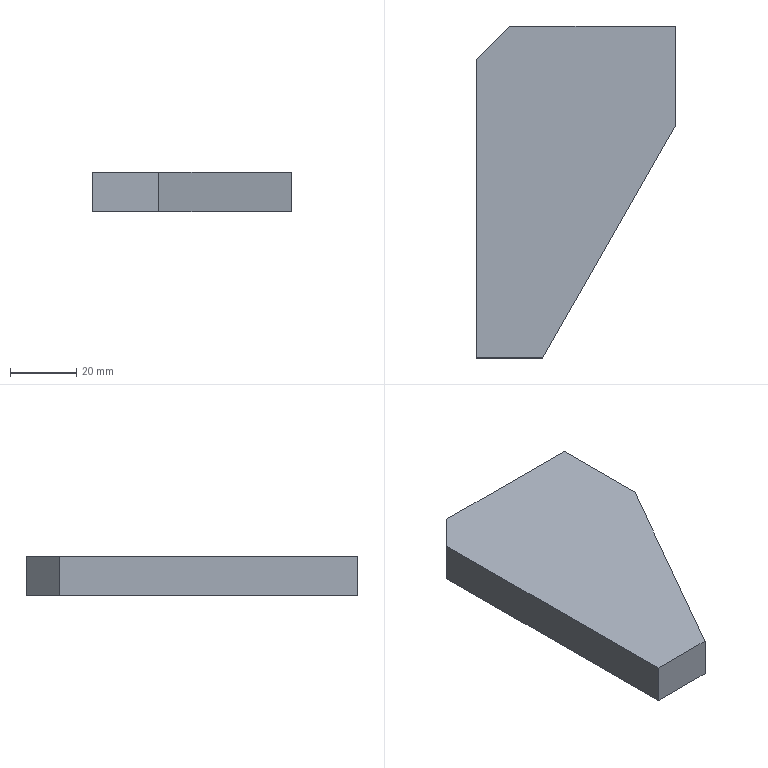Part | STEP file | Gusset plate 1_Default<As machined> | 1 solid | 8 faces | box 60 x 100 x 12 mm | volume 54600 mm3 | plane 8
STEP:
#1=CARTESIAN_POINT('',(0.,0.,0.));
#2=DIRECTION('',(0.,0.,1.));
#3=DIRECTION('',(1.,0.,0.));
#4=AXIS2_PLACEMENT_3D('',#1,#2,#3);
#5=CARTESIAN_POINT('',(0.,-100.,-6.));
#6=VERTEX_POINT('',#5);
#7=CARTESIAN_POINT('',(20.,-100.,-6.));
#8=VERTEX_POINT('',#7);
#9=CARTESIAN_POINT('',(0.,-100.,-6.));
#10=DIRECTION('',(1.,0.,0.));
#11=VECTOR('',#10,1.);
#12=LINE('',#9,#11);
#13=CARTESIAN_POINT('',(0.,-100.,6.));
#14=DIRECTION('',(0.,1.,0.));
#15=DIRECTION('',(0.,0.,1.));
#16=AXIS2_PLACEMENT_3D('',#13,#14,#15);
#17=PLANE('',#16);
#18=CARTESIAN_POINT('',(-12.,0.));
#19=DIRECTION('',(0.,1.));
#20=VECTOR('',#19,1.);
#21=LINE('',#18,#20);
#22=(GEOMETRIC_REPRESENTATION_CONTEXT(2)PARAMETRIC_REPRESENTATION_CONTEXT()REPRESENTATION_CONTEXT('',''));
#23=DEFINITIONAL_REPRESENTATION('',(#21),#22);
#24=PCURVE('',#17,#23);
#25=CARTESIAN_POINT('',(0.,0.,-6.));
#26=DIRECTION('',(0.,0.,1.));
#27=DIRECTION('',(1.,0.,0.));
#28=AXIS2_PLACEMENT_3D('',#25,#26,#27);
#29=PLANE('',#28);
#30=CARTESIAN_POINT('',(0.,-100.));
#31=DIRECTION('',(1.,0.));
#32=VECTOR('',#31,1.);
#33=LINE('',#30,#32);
#34=(GEOMETRIC_REPRESENTATION_CONTEXT(2)PARAMETRIC_REPRESENTATION_CONTEXT()REPRESENTATION_CONTEXT('',''));
#35=DEFINITIONAL_REPRESENTATION('',(#33),#34);
#36=PCURVE('',#29,#35);
#37=SURFACE_CURVE('',#12,(#24,#36),.PCURVE_S1.);
#38=EDGE_CURVE('',#6,#8,#37,.T.);
#39=ORIENTED_EDGE('',*,*,#38,.T.);
#40=CARTESIAN_POINT('',(20.,-100.,6.));
#41=VERTEX_POINT('',#40);
#42=CARTESIAN_POINT('',(20.,-100.,6.));
#43=DIRECTION('',(0.,0.,-1.));
#44=VECTOR('',#43,1.);
#45=LINE('',#42,#44);
#46=CARTESIAN_POINT('',(0.,20.));
#47=DIRECTION('',(-1.,0.));
#48=VECTOR('',#47,1.);
#49=LINE('',#46,#48);
#50=(GEOMETRIC_REPRESENTATION_CONTEXT(2)PARAMETRIC_REPRESENTATION_CONTEXT()REPRESENTATION_CONTEXT('',''));
#51=DEFINITIONAL_REPRESENTATION('',(#49),#50);
#52=PCURVE('',#17,#51);
#53=CARTESIAN_POINT('',(20.,-100.,6.));
#54=DIRECTION('',(-0.8682,0.4961,0.));
#55=DIRECTION('',(-0.4961,-0.8682,0.));
#56=AXIS2_PLACEMENT_3D('',#53,#54,#55);
#57=PLANE('',#56);
#58=CARTESIAN_POINT('',(0.,0.));
#59=DIRECTION('',(0.,-1.));
#60=VECTOR('',#59,1.);
#61=LINE('',#58,#60);
#62=(GEOMETRIC_REPRESENTATION_CONTEXT(2)PARAMETRIC_REPRESENTATION_CONTEXT()REPRESENTATION_CONTEXT('',''));
#63=DEFINITIONAL_REPRESENTATION('',(#61),#62);
#64=PCURVE('',#57,#63);
#65=SURFACE_CURVE('',#45,(#52,#64),.PCURVE_S1.);
#66=EDGE_CURVE('',#41,#8,#65,.T.);
#67=ORIENTED_EDGE('',*,*,#66,.F.);
#68=CARTESIAN_POINT('',(0.,-100.,6.));
#69=VERTEX_POINT('',#68);
#70=CARTESIAN_POINT('',(0.,-100.,6.));
#71=DIRECTION('',(1.,0.,0.));
#72=VECTOR('',#71,1.);
#73=LINE('',#70,#72);
#74=CARTESIAN_POINT('',(0.,0.));
#75=DIRECTION('',(0.,1.));
#76=VECTOR('',#75,1.);
#77=LINE('',#74,#76);
#78=(GEOMETRIC_REPRESENTATION_CONTEXT(2)PARAMETRIC_REPRESENTATION_CONTEXT()REPRESENTATION_CONTEXT('',''));
#79=DEFINITIONAL_REPRESENTATION('',(#77),#78);
#80=PCURVE('',#17,#79);
#81=CARTESIAN_POINT('',(0.,0.,6.));
#82=DIRECTION('',(0.,0.,1.));
#83=DIRECTION('',(1.,0.,0.));
#84=AXIS2_PLACEMENT_3D('',#81,#82,#83);
#85=PLANE('',#84);
#86=CARTESIAN_POINT('',(0.,-100.));
#87=DIRECTION('',(1.,0.));
#88=VECTOR('',#87,1.);
#89=LINE('',#86,#88);
#90=(GEOMETRIC_REPRESENTATION_CONTEXT(2)PARAMETRIC_REPRESENTATION_CONTEXT()REPRESENTATION_CONTEXT('',''));
#91=DEFINITIONAL_REPRESENTATION('',(#89),#90);
#92=PCURVE('',#85,#91);
#93=SURFACE_CURVE('',#73,(#80,#92),.PCURVE_S1.);
#94=EDGE_CURVE('',#69,#41,#93,.T.);
#95=ORIENTED_EDGE('',*,*,#94,.F.);
#96=CARTESIAN_POINT('',(0.,-100.,6.));
#97=DIRECTION('',(0.,0.,-1.));
#98=VECTOR('',#97,1.);
#99=LINE('',#96,#98);
#100=CARTESIAN_POINT('',(0.,0.));
#101=DIRECTION('',(-1.,0.));
#102=VECTOR('',#101,1.);
#103=LINE('',#100,#102);
#104=(GEOMETRIC_REPRESENTATION_CONTEXT(2)PARAMETRIC_REPRESENTATION_CONTEXT()REPRESENTATION_CONTEXT('',''));
#105=DEFINITIONAL_REPRESENTATION('',(#103),#104);
#106=PCURVE('',#17,#105);
#107=CARTESIAN_POINT('',(0.,-10.,6.));
#108=DIRECTION('',(1.,0.,0.));
#109=DIRECTION('',(0.,1.,0.));
#110=AXIS2_PLACEMENT_3D('',#107,#108,#109);
#111=PLANE('',#110);
#112=CARTESIAN_POINT('',(-90.,0.));
#113=DIRECTION('',(0.,-1.));
#114=VECTOR('',#113,1.);
#115=LINE('',#112,#114);
#116=(GEOMETRIC_REPRESENTATION_CONTEXT(2)PARAMETRIC_REPRESENTATION_CONTEXT()REPRESENTATION_CONTEXT('',''));
#117=DEFINITIONAL_REPRESENTATION('',(#115),#116);
#118=PCURVE('',#111,#117);
#119=SURFACE_CURVE('',#99,(#106,#118),.PCURVE_S1.);
#120=EDGE_CURVE('',#69,#6,#119,.T.);
#121=ORIENTED_EDGE('',*,*,#120,.T.);
#122=EDGE_LOOP('',(#39,#67,#95,#121));
#123=FACE_BOUND('',#122,.T.);
#124=ADVANCED_FACE('',(#123),#17,.F.);
#125=CARTESIAN_POINT('',(60.,-30.,-6.));
#126=VERTEX_POINT('',#125);
#127=CARTESIAN_POINT('',(20.,-100.,-6.));
#128=DIRECTION('',(0.4961,0.8682,0.));
#129=VECTOR('',#128,1.);
#130=LINE('',#127,#129);
#131=CARTESIAN_POINT('',(0.,-12.));
#132=DIRECTION('',(-1.,0.));
#133=VECTOR('',#132,1.);
#134=LINE('',#131,#133);
#135=(GEOMETRIC_REPRESENTATION_CONTEXT(2)PARAMETRIC_REPRESENTATION_CONTEXT()REPRESENTATION_CONTEXT('',''));
#136=DEFINITIONAL_REPRESENTATION('',(#134),#135);
#137=PCURVE('',#57,#136);
#138=CARTESIAN_POINT('',(20.,-100.));
#139=DIRECTION('',(0.4961,0.8682));
#140=VECTOR('',#139,1.);
#141=LINE('',#138,#140);
#142=(GEOMETRIC_REPRESENTATION_CONTEXT(2)PARAMETRIC_REPRESENTATION_CONTEXT()REPRESENTATION_CONTEXT('',''));
#143=DEFINITIONAL_REPRESENTATION('',(#141),#142);
#144=PCURVE('',#29,#143);
#145=SURFACE_CURVE('',#130,(#137,#144),.PCURVE_S1.);
#146=EDGE_CURVE('',#8,#126,#145,.T.);
#147=ORIENTED_EDGE('',*,*,#146,.T.);
#148=CARTESIAN_POINT('',(60.,-30.,6.));
#149=VERTEX_POINT('',#148);
#150=CARTESIAN_POINT('',(60.,-30.,6.));
#151=DIRECTION('',(0.,0.,-1.));
#152=VECTOR('',#151,1.);
#153=LINE('',#150,#152);
#154=CARTESIAN_POINT('',(-80.623,0.));
#155=DIRECTION('',(0.,-1.));
#156=VECTOR('',#155,1.);
#157=LINE('',#154,#156);
#158=(GEOMETRIC_REPRESENTATION_CONTEXT(2)PARAMETRIC_REPRESENTATION_CONTEXT()REPRESENTATION_CONTEXT('',''));
#159=DEFINITIONAL_REPRESENTATION('',(#157),#158);
#160=PCURVE('',#57,#159);
#161=CARTESIAN_POINT('',(60.,-30.,6.));
#162=DIRECTION('',(-1.,0.,0.));
#163=DIRECTION('',(0.,0.,1.));
#164=AXIS2_PLACEMENT_3D('',#161,#162,#163);
#165=PLANE('',#164);
#166=CARTESIAN_POINT('',(0.,0.));
#167=DIRECTION('',(-1.,0.));
#168=VECTOR('',#167,1.);
#169=LINE('',#166,#168);
#170=(GEOMETRIC_REPRESENTATION_CONTEXT(2)PARAMETRIC_REPRESENTATION_CONTEXT()REPRESENTATION_CONTEXT('',''));
#171=DEFINITIONAL_REPRESENTATION('',(#169),#170);
#172=PCURVE('',#165,#171);
#173=SURFACE_CURVE('',#153,(#160,#172),.PCURVE_S1.);
#174=EDGE_CURVE('',#149,#126,#173,.T.);
#175=ORIENTED_EDGE('',*,*,#174,.F.);
#176=CARTESIAN_POINT('',(20.,-100.,6.));
#177=DIRECTION('',(0.4961,0.8682,0.));
#178=VECTOR('',#177,1.);
#179=LINE('',#176,#178);
#180=CARTESIAN_POINT('',(0.,0.));
#181=DIRECTION('',(-1.,0.));
#182=VECTOR('',#181,1.);
#183=LINE('',#180,#182);
#184=(GEOMETRIC_REPRESENTATION_CONTEXT(2)PARAMETRIC_REPRESENTATION_CONTEXT()REPRESENTATION_CONTEXT('',''));
#185=DEFINITIONAL_REPRESENTATION('',(#183),#184);
#186=PCURVE('',#57,#185);
#187=CARTESIAN_POINT('',(20.,-100.));
#188=DIRECTION('',(0.4961,0.8682));
#189=VECTOR('',#188,1.);
#190=LINE('',#187,#189);
#191=(GEOMETRIC_REPRESENTATION_CONTEXT(2)PARAMETRIC_REPRESENTATION_CONTEXT()REPRESENTATION_CONTEXT('',''));
#192=DEFINITIONAL_REPRESENTATION('',(#190),#191);
#193=PCURVE('',#85,#192);
#194=SURFACE_CURVE('',#179,(#186,#193),.PCURVE_S1.);
#195=EDGE_CURVE('',#41,#149,#194,.T.);
#196=ORIENTED_EDGE('',*,*,#195,.F.);
#197=ORIENTED_EDGE('',*,*,#66,.T.);
#198=EDGE_LOOP('',(#147,#175,#196,#197));
#199=FACE_BOUND('',#198,.T.);
#200=ADVANCED_FACE('',(#199),#57,.F.);
#201=CARTESIAN_POINT('',(60.,0.,-6.));
#202=VERTEX_POINT('',#201);
#203=CARTESIAN_POINT('',(60.,-30.,-6.));
#204=DIRECTION('',(0.,1.,0.));
#205=VECTOR('',#204,1.);
#206=LINE('',#203,#205);
#207=CARTESIAN_POINT('',(-12.,0.));
#208=DIRECTION('',(0.,1.));
#209=VECTOR('',#208,1.);
#210=LINE('',#207,#209);
#211=(GEOMETRIC_REPRESENTATION_CONTEXT(2)PARAMETRIC_REPRESENTATION_CONTEXT()REPRESENTATION_CONTEXT('',''));
#212=DEFINITIONAL_REPRESENTATION('',(#210),#211);
#213=PCURVE('',#165,#212);
#214=CARTESIAN_POINT('',(60.,-30.));
#215=DIRECTION('',(0.,1.));
#216=VECTOR('',#215,1.);
#217=LINE('',#214,#216);
#218=(GEOMETRIC_REPRESENTATION_CONTEXT(2)PARAMETRIC_REPRESENTATION_CONTEXT()REPRESENTATION_CONTEXT('',''));
#219=DEFINITIONAL_REPRESENTATION('',(#217),#218);
#220=PCURVE('',#29,#219);
#221=SURFACE_CURVE('',#206,(#213,#220),.PCURVE_S1.);
#222=EDGE_CURVE('',#126,#202,#221,.T.);
#223=ORIENTED_EDGE('',*,*,#222,.T.);
#224=CARTESIAN_POINT('',(60.,0.,6.));
#225=VERTEX_POINT('',#224);
#226=CARTESIAN_POINT('',(60.,0.,6.));
#227=DIRECTION('',(0.,0.,-1.));
#228=VECTOR('',#227,1.);
#229=LINE('',#226,#228);
#230=CARTESIAN_POINT('',(0.,30.));
#231=DIRECTION('',(-1.,0.));
#232=VECTOR('',#231,1.);
#233=LINE('',#230,#232);
#234=(GEOMETRIC_REPRESENTATION_CONTEXT(2)PARAMETRIC_REPRESENTATION_CONTEXT()REPRESENTATION_CONTEXT('',''));
#235=DEFINITIONAL_REPRESENTATION('',(#233),#234);
#236=PCURVE('',#165,#235);
#237=CARTESIAN_POINT('',(60.,0.,6.));
#238=DIRECTION('',(0.,-1.,0.));
#239=DIRECTION('',(1.,0.,0.));
#240=AXIS2_PLACEMENT_3D('',#237,#238,#239);
#241=PLANE('',#240);
#242=CARTESIAN_POINT('',(0.,0.));
#243=DIRECTION('',(0.,-1.));
#244=VECTOR('',#243,1.);
#245=LINE('',#242,#244);
#246=(GEOMETRIC_REPRESENTATION_CONTEXT(2)PARAMETRIC_REPRESENTATION_CONTEXT()REPRESENTATION_CONTEXT('',''));
#247=DEFINITIONAL_REPRESENTATION('',(#245),#246);
#248=PCURVE('',#241,#247);
#249=SURFACE_CURVE('',#229,(#236,#248),.PCURVE_S1.);
#250=EDGE_CURVE('',#225,#202,#249,.T.);
#251=ORIENTED_EDGE('',*,*,#250,.F.);
#252=CARTESIAN_POINT('',(60.,-30.,6.));
#253=DIRECTION('',(0.,1.,0.));
#254=VECTOR('',#253,1.);
#255=LINE('',#252,#254);
#256=CARTESIAN_POINT('',(0.,0.));
#257=DIRECTION('',(0.,1.));
#258=VECTOR('',#257,1.);
#259=LINE('',#256,#258);
#260=(GEOMETRIC_REPRESENTATION_CONTEXT(2)PARAMETRIC_REPRESENTATION_CONTEXT()REPRESENTATION_CONTEXT('',''));
#261=DEFINITIONAL_REPRESENTATION('',(#259),#260);
#262=PCURVE('',#165,#261);
#263=CARTESIAN_POINT('',(60.,-30.));
#264=DIRECTION('',(0.,1.));
#265=VECTOR('',#264,1.);
#266=LINE('',#263,#265);
#267=(GEOMETRIC_REPRESENTATION_CONTEXT(2)PARAMETRIC_REPRESENTATION_CONTEXT()REPRESENTATION_CONTEXT('',''));
#268=DEFINITIONAL_REPRESENTATION('',(#266),#267);
#269=PCURVE('',#85,#268);
#270=SURFACE_CURVE('',#255,(#262,#269),.PCURVE_S1.);
#271=EDGE_CURVE('',#149,#225,#270,.T.);
#272=ORIENTED_EDGE('',*,*,#271,.F.);
#273=ORIENTED_EDGE('',*,*,#174,.T.);
#274=EDGE_LOOP('',(#223,#251,#272,#273));
#275=FACE_BOUND('',#274,.T.);
#276=ADVANCED_FACE('',(#275),#165,.F.);
#277=CARTESIAN_POINT('',(10.,0.,-6.));
#278=VERTEX_POINT('',#277);
#279=CARTESIAN_POINT('',(60.,0.,-6.));
#280=DIRECTION('',(-1.,0.,0.));
#281=VECTOR('',#280,1.);
#282=LINE('',#279,#281);
#283=CARTESIAN_POINT('',(0.,-12.));
#284=DIRECTION('',(-1.,0.));
#285=VECTOR('',#284,1.);
#286=LINE('',#283,#285);
#287=(GEOMETRIC_REPRESENTATION_CONTEXT(2)PARAMETRIC_REPRESENTATION_CONTEXT()REPRESENTATION_CONTEXT('',''));
#288=DEFINITIONAL_REPRESENTATION('',(#286),#287);
#289=PCURVE('',#241,#288);
#290=CARTESIAN_POINT('',(60.,0.));
#291=DIRECTION('',(-1.,0.));
#292=VECTOR('',#291,1.);
#293=LINE('',#290,#292);
#294=(GEOMETRIC_REPRESENTATION_CONTEXT(2)PARAMETRIC_REPRESENTATION_CONTEXT()REPRESENTATION_CONTEXT('',''));
#295=DEFINITIONAL_REPRESENTATION('',(#293),#294);
#296=PCURVE('',#29,#295);
#297=SURFACE_CURVE('',#282,(#289,#296),.PCURVE_S1.);
#298=EDGE_CURVE('',#202,#278,#297,.T.);
#299=ORIENTED_EDGE('',*,*,#298,.T.);
#300=CARTESIAN_POINT('',(10.,0.,6.));
#301=VERTEX_POINT('',#300);
#302=CARTESIAN_POINT('',(10.,0.,6.));
#303=DIRECTION('',(0.,0.,-1.));
#304=VECTOR('',#303,1.);
#305=LINE('',#302,#304);
#306=CARTESIAN_POINT('',(-50.,0.));
#307=DIRECTION('',(0.,-1.));
#308=VECTOR('',#307,1.);
#309=LINE('',#306,#308);
#310=(GEOMETRIC_REPRESENTATION_CONTEXT(2)PARAMETRIC_REPRESENTATION_CONTEXT()REPRESENTATION_CONTEXT('',''));
#311=DEFINITIONAL_REPRESENTATION('',(#309),#310);
#312=PCURVE('',#241,#311);
#313=CARTESIAN_POINT('',(10.,0.,6.));
#314=DIRECTION('',(0.7071,-0.7071,0.));
#315=DIRECTION('',(0.7071,0.7071,0.));
#316=AXIS2_PLACEMENT_3D('',#313,#314,#315);
#317=PLANE('',#316);
#318=CARTESIAN_POINT('',(0.,0.));
#319=DIRECTION('',(0.,-1.));
#320=VECTOR('',#319,1.);
#321=LINE('',#318,#320);
#322=(GEOMETRIC_REPRESENTATION_CONTEXT(2)PARAMETRIC_REPRESENTATION_CONTEXT()REPRESENTATION_CONTEXT('',''));
#323=DEFINITIONAL_REPRESENTATION('',(#321),#322);
#324=PCURVE('',#317,#323);
#325=SURFACE_CURVE('',#305,(#312,#324),.PCURVE_S1.);
#326=EDGE_CURVE('',#301,#278,#325,.T.);
#327=ORIENTED_EDGE('',*,*,#326,.F.);
#328=CARTESIAN_POINT('',(60.,0.,6.));
#329=DIRECTION('',(-1.,0.,0.));
#330=VECTOR('',#329,1.);
#331=LINE('',#328,#330);
#332=CARTESIAN_POINT('',(0.,0.));
#333=DIRECTION('',(-1.,0.));
#334=VECTOR('',#333,1.);
#335=LINE('',#332,#334);
#336=(GEOMETRIC_REPRESENTATION_CONTEXT(2)PARAMETRIC_REPRESENTATION_CONTEXT()REPRESENTATION_CONTEXT('',''));
#337=DEFINITIONAL_REPRESENTATION('',(#335),#336);
#338=PCURVE('',#241,#337);
#339=CARTESIAN_POINT('',(60.,0.));
#340=DIRECTION('',(-1.,0.));
#341=VECTOR('',#340,1.);
#342=LINE('',#339,#341);
#343=(GEOMETRIC_REPRESENTATION_CONTEXT(2)PARAMETRIC_REPRESENTATION_CONTEXT()REPRESENTATION_CONTEXT('',''));
#344=DEFINITIONAL_REPRESENTATION('',(#342),#343);
#345=PCURVE('',#85,#344);
#346=SURFACE_CURVE('',#331,(#338,#345),.PCURVE_S1.);
#347=EDGE_CURVE('',#225,#301,#346,.T.);
#348=ORIENTED_EDGE('',*,*,#347,.F.);
#349=ORIENTED_EDGE('',*,*,#250,.T.);
#350=EDGE_LOOP('',(#299,#327,#348,#349));
#351=FACE_BOUND('',#350,.T.);
#352=ADVANCED_FACE('',(#351),#241,.F.);
#353=CARTESIAN_POINT('',(0.,-10.,-6.));
#354=VERTEX_POINT('',#353);
#355=CARTESIAN_POINT('',(10.,0.,-6.));
#356=DIRECTION('',(-0.7071,-0.7071,0.));
#357=VECTOR('',#356,1.);
#358=LINE('',#355,#357);
#359=CARTESIAN_POINT('',(0.,-12.));
#360=DIRECTION('',(-1.,0.));
#361=VECTOR('',#360,1.);
#362=LINE('',#359,#361);
#363=(GEOMETRIC_REPRESENTATION_CONTEXT(2)PARAMETRIC_REPRESENTATION_CONTEXT()REPRESENTATION_CONTEXT('',''));
#364=DEFINITIONAL_REPRESENTATION('',(#362),#363);
#365=PCURVE('',#317,#364);
#366=CARTESIAN_POINT('',(10.,0.));
#367=DIRECTION('',(-0.7071,-0.7071));
#368=VECTOR('',#367,1.);
#369=LINE('',#366,#368);
#370=(GEOMETRIC_REPRESENTATION_CONTEXT(2)PARAMETRIC_REPRESENTATION_CONTEXT()REPRESENTATION_CONTEXT('',''));
#371=DEFINITIONAL_REPRESENTATION('',(#369),#370);
#372=PCURVE('',#29,#371);
#373=SURFACE_CURVE('',#358,(#365,#372),.PCURVE_S1.);
#374=EDGE_CURVE('',#278,#354,#373,.T.);
#375=ORIENTED_EDGE('',*,*,#374,.T.);
#376=CARTESIAN_POINT('',(0.,-10.,6.));
#377=VERTEX_POINT('',#376);
#378=CARTESIAN_POINT('',(0.,-10.,6.));
#379=DIRECTION('',(0.,0.,-1.));
#380=VECTOR('',#379,1.);
#381=LINE('',#378,#380);
#382=CARTESIAN_POINT('',(-14.142,0.));
#383=DIRECTION('',(0.,-1.));
#384=VECTOR('',#383,1.);
#385=LINE('',#382,#384);
#386=(GEOMETRIC_REPRESENTATION_CONTEXT(2)PARAMETRIC_REPRESENTATION_CONTEXT()REPRESENTATION_CONTEXT('',''));
#387=DEFINITIONAL_REPRESENTATION('',(#385),#386);
#388=PCURVE('',#317,#387);
#389=CARTESIAN_POINT('',(0.,0.));
#390=DIRECTION('',(0.,-1.));
#391=VECTOR('',#390,1.);
#392=LINE('',#389,#391);
#393=(GEOMETRIC_REPRESENTATION_CONTEXT(2)PARAMETRIC_REPRESENTATION_CONTEXT()REPRESENTATION_CONTEXT('',''));
#394=DEFINITIONAL_REPRESENTATION('',(#392),#393);
#395=PCURVE('',#111,#394);
#396=SURFACE_CURVE('',#381,(#388,#395),.PCURVE_S1.);
#397=EDGE_CURVE('',#377,#354,#396,.T.);
#398=ORIENTED_EDGE('',*,*,#397,.F.);
#399=CARTESIAN_POINT('',(10.,0.,6.));
#400=DIRECTION('',(-0.7071,-0.7071,0.));
#401=VECTOR('',#400,1.);
#402=LINE('',#399,#401);
#403=CARTESIAN_POINT('',(0.,0.));
#404=DIRECTION('',(-1.,0.));
#405=VECTOR('',#404,1.);
#406=LINE('',#403,#405);
#407=(GEOMETRIC_REPRESENTATION_CONTEXT(2)PARAMETRIC_REPRESENTATION_CONTEXT()REPRESENTATION_CONTEXT('',''));
#408=DEFINITIONAL_REPRESENTATION('',(#406),#407);
#409=PCURVE('',#317,#408);
#410=CARTESIAN_POINT('',(10.,0.));
#411=DIRECTION('',(-0.7071,-0.7071));
#412=VECTOR('',#411,1.);
#413=LINE('',#410,#412);
#414=(GEOMETRIC_REPRESENTATION_CONTEXT(2)PARAMETRIC_REPRESENTATION_CONTEXT()REPRESENTATION_CONTEXT('',''));
#415=DEFINITIONAL_REPRESENTATION('',(#413),#414);
#416=PCURVE('',#85,#415);
#417=SURFACE_CURVE('',#402,(#409,#416),.PCURVE_S1.);
#418=EDGE_CURVE('',#301,#377,#417,.T.);
#419=ORIENTED_EDGE('',*,*,#418,.F.);
#420=ORIENTED_EDGE('',*,*,#326,.T.);
#421=EDGE_LOOP('',(#375,#398,#419,#420));
#422=FACE_BOUND('',#421,.T.);
#423=ADVANCED_FACE('',(#422),#317,.F.);
#424=CARTESIAN_POINT('',(0.,-10.,-6.));
#425=DIRECTION('',(0.,-1.,0.));
#426=VECTOR('',#425,1.);
#427=LINE('',#424,#426);
#428=CARTESIAN_POINT('',(0.,-12.));
#429=DIRECTION('',(-1.,0.));
#430=VECTOR('',#429,1.);
#431=LINE('',#428,#430);
#432=(GEOMETRIC_REPRESENTATION_CONTEXT(2)PARAMETRIC_REPRESENTATION_CONTEXT()REPRESENTATION_CONTEXT('',''));
#433=DEFINITIONAL_REPRESENTATION('',(#431),#432);
#434=PCURVE('',#111,#433);
#435=CARTESIAN_POINT('',(0.,-10.));
#436=DIRECTION('',(0.,-1.));
#437=VECTOR('',#436,1.);
#438=LINE('',#435,#437);
#439=(GEOMETRIC_REPRESENTATION_CONTEXT(2)PARAMETRIC_REPRESENTATION_CONTEXT()REPRESENTATION_CONTEXT('',''));
#440=DEFINITIONAL_REPRESENTATION('',(#438),#439);
#441=PCURVE('',#29,#440);
#442=SURFACE_CURVE('',#427,(#434,#441),.PCURVE_S1.);
#443=EDGE_CURVE('',#354,#6,#442,.T.);
#444=ORIENTED_EDGE('',*,*,#443,.T.);
#445=ORIENTED_EDGE('',*,*,#120,.F.);
#446=CARTESIAN_POINT('',(0.,-10.,6.));
#447=DIRECTION('',(0.,-1.,0.));
#448=VECTOR('',#447,1.);
#449=LINE('',#446,#448);
#450=CARTESIAN_POINT('',(0.,0.));
#451=DIRECTION('',(-1.,0.));
#452=VECTOR('',#451,1.);
#453=LINE('',#450,#452);
#454=(GEOMETRIC_REPRESENTATION_CONTEXT(2)PARAMETRIC_REPRESENTATION_CONTEXT()REPRESENTATION_CONTEXT('',''));
#455=DEFINITIONAL_REPRESENTATION('',(#453),#454);
#456=PCURVE('',#111,#455);
#457=CARTESIAN_POINT('',(0.,-10.));
#458=DIRECTION('',(0.,-1.));
#459=VECTOR('',#458,1.);
#460=LINE('',#457,#459);
#461=(GEOMETRIC_REPRESENTATION_CONTEXT(2)PARAMETRIC_REPRESENTATION_CONTEXT()REPRESENTATION_CONTEXT('',''));
#462=DEFINITIONAL_REPRESENTATION('',(#460),#461);
#463=PCURVE('',#85,#462);
#464=SURFACE_CURVE('',#449,(#456,#463),.PCURVE_S1.);
#465=EDGE_CURVE('',#377,#69,#464,.T.);
#466=ORIENTED_EDGE('',*,*,#465,.F.);
#467=ORIENTED_EDGE('',*,*,#397,.T.);
#468=EDGE_LOOP('',(#444,#445,#466,#467));
#469=FACE_BOUND('',#468,.T.);
#470=ADVANCED_FACE('',(#469),#111,.F.);
#471=ORIENTED_EDGE('',*,*,#94,.T.);
#472=ORIENTED_EDGE('',*,*,#195,.T.);
#473=ORIENTED_EDGE('',*,*,#271,.T.);
#474=ORIENTED_EDGE('',*,*,#347,.T.);
#475=ORIENTED_EDGE('',*,*,#418,.T.);
#476=ORIENTED_EDGE('',*,*,#465,.T.);
#477=EDGE_LOOP('',(#471,#472,#473,#474,#475,#476));
#478=FACE_BOUND('',#477,.T.);
#479=ADVANCED_FACE('',(#478),#85,.T.);
#480=ORIENTED_EDGE('',*,*,#38,.F.);
#481=ORIENTED_EDGE('',*,*,#443,.F.);
#482=ORIENTED_EDGE('',*,*,#374,.F.);
#483=ORIENTED_EDGE('',*,*,#298,.F.);
#484=ORIENTED_EDGE('',*,*,#222,.F.);
#485=ORIENTED_EDGE('',*,*,#146,.F.);
#486=EDGE_LOOP('',(#480,#481,#482,#483,#484,#485));
#487=FACE_BOUND('',#486,.T.);
#488=ADVANCED_FACE('',(#487),#29,.F.);
#489=CLOSED_SHELL('',(#124,#200,#276,#352,#423,#470,#479,#488));
#490=MANIFOLD_SOLID_BREP('',#489);
#491=(LENGTH_UNIT()NAMED_UNIT(*)SI_UNIT(.MILLI.,.METRE.));
#492=UNCERTAINTY_MEASURE_WITH_UNIT(LENGTH_MEASURE(0.0000001),#491,'','');
#493=(NAMED_UNIT(*)PLANE_ANGLE_UNIT()SI_UNIT($,.RADIAN.));
#494=(NAMED_UNIT(*)SI_UNIT($,.STERADIAN.)SOLID_ANGLE_UNIT());
#495=(GEOMETRIC_REPRESENTATION_CONTEXT(3)GLOBAL_UNCERTAINTY_ASSIGNED_CONTEXT((#492))GLOBAL_UNIT_ASSIGNED_CONTEXT((#491,#493,#494))REPRESENTATION_CONTEXT('',''));
#496=ADVANCED_BREP_SHAPE_REPRESENTATION('',(#4,#490),#495);